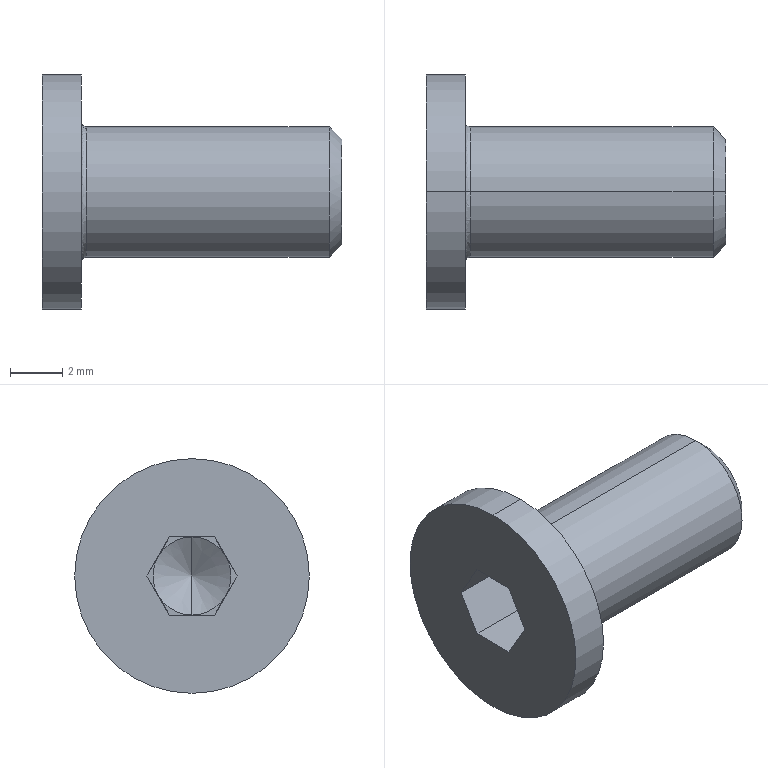Part | STEP file | cbss5_10_2_03 | 1 solid | 25 faces | box 11.5 x 9 x 9 mm | volume 264.715 mm3 | plane 15 | cylinder 4 | cone 4 | spline 2 | commonest cylinder face diameters 5 x2 9 x2